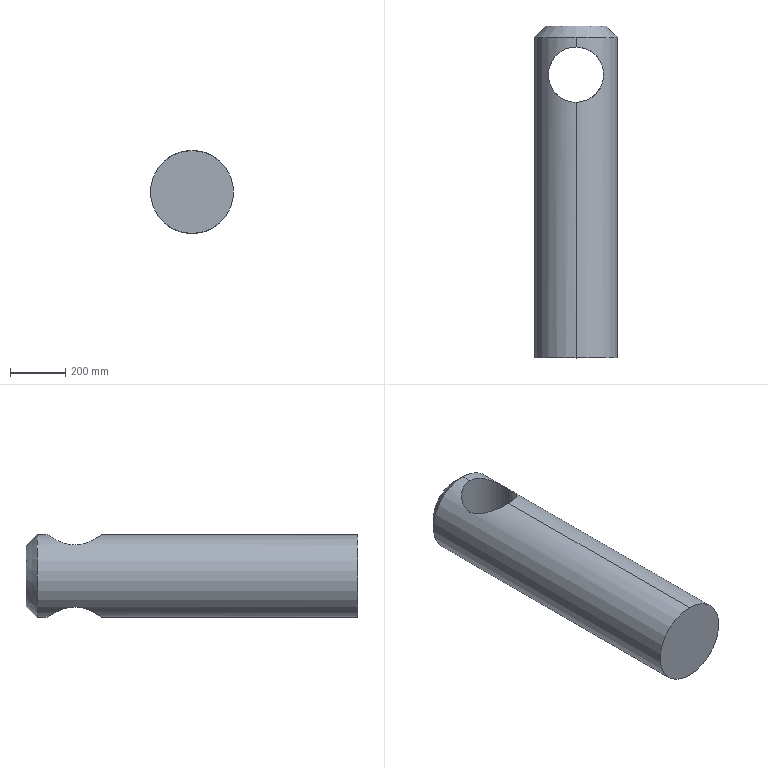Part | SolidWorks | features ICE 2, Chamfer 1, Extrusion 1 | 1 solid | 8 faces | box 300 x 1200 x 300 mm | volume 75269036 mm3 | cylinder 4 | cone 2 | plane 2 | commonest cylinder face diameters 200 x2 300 x2
STEP:
#1=CARTESIAN_POINT('',(0.,2400.,110.));
#2=VERTEX_POINT('',#1);
#3=CARTESIAN_POINT('',(0.,2400.,-110.));
#4=VERTEX_POINT('',#3);
#5=CARTESIAN_POINT('',(0.,2400.,0.));
#6=DIRECTION('',(0.,1.,0.));
#7=DIRECTION('',(0.,0.,1.));
#8=AXIS2_PLACEMENT_3D('',#5,#6,#7);
#9=CIRCLE('',#8,110.);
#10=EDGE_CURVE('',#2,#4,#9,.T.);
#11=ORIENTED_EDGE('',*,*,#10,.F.);
#12=CARTESIAN_POINT('',(0.,2360.,150.));
#13=VERTEX_POINT('',#12);
#14=CARTESIAN_POINT('',(0.,2400.,110.));
#15=DIRECTION('',(0.,-0.7071,0.7071));
#16=VECTOR('',#15,1000.);
#17=LINE('',#14,#16);
#18=EDGE_CURVE('',#2,#13,#17,.T.);
#19=ORIENTED_EDGE('',*,*,#18,.T.);
#20=CARTESIAN_POINT('',(0.,2360.,-150.));
#21=VERTEX_POINT('',#20);
#22=CARTESIAN_POINT('',(0.,2360.,0.));
#23=DIRECTION('',(0.,-1.,0.));
#24=DIRECTION('',(0.,0.,1.));
#25=AXIS2_PLACEMENT_3D('',#22,#23,#24);
#26=CIRCLE('',#25,150.);
#27=EDGE_CURVE('',#21,#13,#26,.T.);
#28=ORIENTED_EDGE('',*,*,#27,.F.);
#29=CARTESIAN_POINT('',(0.,2400.,-110.));
#30=DIRECTION('',(0.,-0.7071,-0.7071));
#31=VECTOR('',#30,1000.);
#32=LINE('',#29,#31);
#33=EDGE_CURVE('',#4,#21,#32,.T.);
#34=ORIENTED_EDGE('',*,*,#33,.F.);
#35=EDGE_LOOP('',(#11,#19,#28,#34));
#36=FACE_OUTER_BOUND('',#35,.T.);
#37=CARTESIAN_POINT('',(0.,2400.,0.));
#38=DIRECTION('',(0.,-1.,0.));
#39=DIRECTION('',(0.,0.,-1.));
#40=AXIS2_PLACEMENT_3D('',#37,#38,#39);
#41=CONICAL_SURFACE('',#40,110.,0.7854);
#42=ADVANCED_FACE('',(#36),#41,.T.);
#43=CARTESIAN_POINT('',(0.,2124.224,150.));
#44=VERTEX_POINT('',#43);
#45=CARTESIAN_POINT('',(100.,2224.224,111.803));
#46=VERTEX_POINT('',#45);
#47=CARTESIAN_POINT('',(0.,2124.224,150.));
#48=CARTESIAN_POINT('',(0.8516,2124.224,150.));
#49=CARTESIAN_POINT('',(1.707,2124.235,149.993));
#50=CARTESIAN_POINT('',(3.415,2124.278,149.964));
#51=CARTESIAN_POINT('',(4.266,2124.311,149.942));
#52=CARTESIAN_POINT('',(6.812,2124.441,149.855));
#53=CARTESIAN_POINT('',(8.499,2124.571,149.768));
#54=CARTESIAN_POINT('',(13.531,2125.086,149.426));
#55=CARTESIAN_POINT('',(16.847,2125.596,149.088));
#56=CARTESIAN_POINT('',(23.402,2126.943,148.2));
#57=CARTESIAN_POINT('',(26.641,2127.779,147.651));
#58=CARTESIAN_POINT('',(31.443,2129.281,146.676));
#59=CARTESIAN_POINT('',(33.023,2129.819,146.328));
#60=CARTESIAN_POINT('',(36.134,2130.965,145.592));
#61=CARTESIAN_POINT('',(37.666,2131.574,145.202));
#62=CARTESIAN_POINT('',(42.196,2133.503,143.977));
#63=CARTESIAN_POINT('',(45.127,2134.926,143.082));
#64=CARTESIAN_POINT('',(49.399,2137.262,141.64));
#65=CARTESIAN_POINT('',(50.802,2138.074,141.143));
#66=CARTESIAN_POINT('',(52.876,2139.342,140.374));
#67=CARTESIAN_POINT('',(53.562,2139.774,140.113));
#68=CARTESIAN_POINT('',(54.923,2140.653,139.585));
#69=CARTESIAN_POINT('',(55.599,2141.101,139.317));
#70=CARTESIAN_POINT('',(58.939,2143.374,137.966));
#71=CARTESIAN_POINT('',(61.492,2145.301,136.843));
#72=CARTESIAN_POINT('',(66.379,2149.365,134.54));
#73=CARTESIAN_POINT('',(68.713,2151.501,133.36));
#74=CARTESIAN_POINT('',(73.171,2155.989,130.967));
#75=CARTESIAN_POINT('',(75.295,2158.339,129.754));
#76=CARTESIAN_POINT('',(78.326,2162.034,127.931));
#77=CARTESIAN_POINT('',(79.306,2163.289,127.326));
#78=CARTESIAN_POINT('',(81.199,2165.835,126.127));
#79=CARTESIAN_POINT('',(82.114,2167.129,125.533));
#80=CARTESIAN_POINT('',(84.762,2171.069,123.774));
#81=CARTESIAN_POINT('',(86.402,2173.777,122.631));
#82=CARTESIAN_POINT('',(89.431,2179.366,120.439));
#83=CARTESIAN_POINT('',(90.821,2182.248,119.39));
#84=CARTESIAN_POINT('',(92.713,2186.715,117.919));
#85=CARTESIAN_POINT('',(93.312,2188.229,117.446));
#86=CARTESIAN_POINT('',(94.442,2191.308,116.539));
#87=CARTESIAN_POINT('',(94.975,2192.879,116.104));
#88=CARTESIAN_POINT('',(96.453,2197.619,114.885));
#89=CARTESIAN_POINT('',(97.281,2200.827,114.18));
#90=CARTESIAN_POINT('',(98.622,2207.348,113.024));
#91=CARTESIAN_POINT('',(99.134,2210.66,112.573));
#92=CARTESIAN_POINT('',(99.565,2214.87,112.191));
#93=CARTESIAN_POINT('',(99.641,2215.716,112.123));
#94=CARTESIAN_POINT('',(99.772,2217.415,112.007));
#95=CARTESIAN_POINT('',(99.826,2218.269,111.959));
#96=CARTESIAN_POINT('',(99.957,2220.829,111.842));
#97=CARTESIAN_POINT('',(100.,2222.529,111.803));
#98=CARTESIAN_POINT('',(100.,2224.224,111.803));
#99=B_SPLINE_CURVE_WITH_KNOTS('',3,(#47,#48,#49,#50,#51,#52,#53,#54,#55,#56,#57,#58,#59,#60,#61,#62,#63,#64,#65,#66,#67,#68,#69,#70,#71,#72,#73,#74,#75,#76,#77,#78,#79,#80,#81,#82,#83,#84,#85,#86,#87,#88,#89,#90,#91,#92,#93,#94,#95,#96,#97,#98),.UNSPECIFIED.,.F.,.F.,(4,2,2,2,2,2,2,2,2,2,2,2,2,2,2,2,2,2,2,2,2,2,2,2,2,4),(0.1618,0.1643,0.1668,0.1718,0.1819,0.192,0.197,0.2021,0.2121,0.2172,0.2197,0.2222,0.2323,0.2424,0.2524,0.2575,0.2625,0.2726,0.2827,0.2877,0.2928,0.3028,0.3129,0.3154,0.3179,0.323),.UNSPECIFIED.);
#100=EDGE_CURVE('',#44,#46,#99,.T.);
#101=ORIENTED_EDGE('',*,*,#100,.T.);
#102=CARTESIAN_POINT('',(100.,2224.224,-111.803));
#103=VERTEX_POINT('',#102);
#104=CARTESIAN_POINT('',(100.,2224.224,4000.));
#105=DIRECTION('',(0.,0.,-1.));
#106=VECTOR('',#105,1000.);
#107=LINE('',#104,#106);
#108=EDGE_CURVE('',#46,#103,#107,.T.);
#109=ORIENTED_EDGE('',*,*,#108,.T.);
#110=CARTESIAN_POINT('',(0.,2124.224,-150.));
#111=VERTEX_POINT('',#110);
#112=CARTESIAN_POINT('',(100.,2224.224,-111.803));
#113=CARTESIAN_POINT('',(100.,2220.834,-111.803));
#114=CARTESIAN_POINT('',(99.828,2217.468,-111.958));
#115=CARTESIAN_POINT('',(99.15,2210.785,-112.559));
#116=CARTESIAN_POINT('',(98.643,2207.467,-113.006));
#117=CARTESIAN_POINT('',(97.8,2203.348,-113.733));
#118=CARTESIAN_POINT('',(97.621,2202.525,-113.887));
#119=CARTESIAN_POINT('',(97.244,2200.892,-114.209));
#120=CARTESIAN_POINT('',(97.045,2200.08,-114.378));
#121=CARTESIAN_POINT('',(96.422,2197.662,-114.904));
#122=CARTESIAN_POINT('',(95.97,2196.072,-115.283));
#123=CARTESIAN_POINT('',(94.502,2191.358,-116.494));
#124=CARTESIAN_POINT('',(93.379,2188.294,-117.401));
#125=CARTESIAN_POINT('',(91.483,2183.806,-118.876));
#126=CARTESIAN_POINT('',(90.815,2182.328,-119.388));
#127=CARTESIAN_POINT('',(89.76,2180.136,-120.18));
#128=CARTESIAN_POINT('',(89.4,2179.409,-120.449));
#129=CARTESIAN_POINT('',(88.663,2177.97,-120.992));
#130=CARTESIAN_POINT('',(88.288,2177.256,-121.266));
#131=CARTESIAN_POINT('',(86.371,2173.723,-122.652));
#132=CARTESIAN_POINT('',(84.718,2170.998,-123.804));
#133=CARTESIAN_POINT('',(81.175,2165.736,-126.156));
#134=CARTESIAN_POINT('',(79.284,2163.199,-127.356));
#135=CARTESIAN_POINT('',(76.266,2159.525,-129.17));
#136=CARTESIAN_POINT('',(75.23,2158.322,-129.777));
#137=CARTESIAN_POINT('',(73.095,2155.962,-130.991));
#138=CARTESIAN_POINT('',(71.995,2154.803,-131.599));
#139=CARTESIAN_POINT('',(68.631,2151.423,-133.403));
#140=CARTESIAN_POINT('',(66.291,2149.287,-134.584));
#141=CARTESIAN_POINT('',(61.415,2145.241,-136.878));
#142=CARTESIAN_POINT('',(58.878,2143.331,-137.991));
#143=CARTESIAN_POINT('',(53.596,2139.739,-140.127));
#144=CARTESIAN_POINT('',(50.851,2138.057,-141.15));
#145=CARTESIAN_POINT('',(47.278,2136.102,-142.356));
#146=CARTESIAN_POINT('',(46.557,2135.719,-142.594));
#147=CARTESIAN_POINT('',(45.099,2134.967,-143.062));
#148=CARTESIAN_POINT('',(44.362,2134.598,-143.292));
#149=CARTESIAN_POINT('',(42.139,2133.521,-143.968));
#150=CARTESIAN_POINT('',(40.641,2132.84,-144.398));
#151=CARTESIAN_POINT('',(36.098,2130.908,-145.625));
#152=CARTESIAN_POINT('',(33.004,2129.769,-146.36));
#153=CARTESIAN_POINT('',(26.679,2127.791,-147.644));
#154=CARTESIAN_POINT('',(23.448,2126.953,-148.193));
#155=CARTESIAN_POINT('',(19.319,2126.104,-148.753));
#156=CARTESIAN_POINT('',(18.488,2125.944,-148.859));
#157=CARTESIAN_POINT('',(16.818,2125.644,-149.057));
#158=CARTESIAN_POINT('',(15.977,2125.505,-149.149));
#159=CARTESIAN_POINT('',(13.458,2125.119,-149.405));
#160=CARTESIAN_POINT('',(11.778,2124.905,-149.546));
#161=CARTESIAN_POINT('',(6.735,2124.393,-149.887));
#162=CARTESIAN_POINT('',(3.369,2124.224,-150.));
#163=CARTESIAN_POINT('',(0.,2124.224,-150.));
#164=B_SPLINE_CURVE_WITH_KNOTS('',3,(#112,#113,#114,#115,#116,#117,#118,#119,#120,#121,#122,#123,#124,#125,#126,#127,#128,#129,#130,#131,#132,#133,#134,#135,#136,#137,#138,#139,#140,#141,#142,#143,#144,#145,#146,#147,#148,#149,#150,#151,#152,#153,#154,#155,#156,#157,#158,#159,#160,#161,#162,#163),.UNSPECIFIED.,.F.,.F.,(4,2,2,2,2,2,2,2,2,2,2,2,2,2,2,2,2,2,2,2,2,2,2,2,2,4),(0.1617,0.1718,0.1819,0.1844,0.1869,0.192,0.2021,0.2071,0.2096,0.2122,0.2223,0.2323,0.2374,0.2424,0.2525,0.2626,0.2727,0.2752,0.2778,0.2828,0.2929,0.303,0.3055,0.3081,0.3131,0.3232),.UNSPECIFIED.);
#165=EDGE_CURVE('',#103,#111,#164,.T.);
#166=ORIENTED_EDGE('',*,*,#165,.T.);
#167=CARTESIAN_POINT('',(-100.,2224.224,-111.803));
#168=VERTEX_POINT('',#167);
#169=CARTESIAN_POINT('',(0.,2124.224,-150.));
#170=CARTESIAN_POINT('',(-3.365,2124.224,-150.));
#171=CARTESIAN_POINT('',(-6.734,2124.393,-149.887));
#172=CARTESIAN_POINT('',(-10.949,2124.821,-149.602));
#173=CARTESIAN_POINT('',(-11.792,2124.918,-149.538));
#174=CARTESIAN_POINT('',(-13.479,2125.133,-149.396));
#175=CARTESIAN_POINT('',(-14.324,2125.251,-149.317));
#176=CARTESIAN_POINT('',(-16.84,2125.637,-149.061));
#177=CARTESIAN_POINT('',(-18.501,2125.936,-148.864));
#178=CARTESIAN_POINT('',(-23.436,2126.951,-148.195));
#179=CARTESIAN_POINT('',(-26.662,2127.786,-147.647));
#180=CARTESIAN_POINT('',(-32.993,2129.765,-146.362));
#181=CARTESIAN_POINT('',(-36.097,2130.907,-145.626));
#182=CARTESIAN_POINT('',(-39.904,2132.526,-144.597));
#183=CARTESIAN_POINT('',(-40.662,2132.86,-144.386));
#184=CARTESIAN_POINT('',(-42.164,2133.544,-143.954));
#185=CARTESIAN_POINT('',(-42.908,2133.893,-143.734));
#186=CARTESIAN_POINT('',(-45.121,2134.967,-143.061));
#187=CARTESIAN_POINT('',(-46.57,2135.715,-142.596));
#188=CARTESIAN_POINT('',(-50.841,2138.051,-141.153));
#189=CARTESIAN_POINT('',(-53.588,2139.734,-140.13));
#190=CARTESIAN_POINT('',(-58.893,2143.342,-137.985));
#191=CARTESIAN_POINT('',(-61.451,2145.267,-136.862));
#192=CARTESIAN_POINT('',(-65.15,2148.342,-135.12));
#193=CARTESIAN_POINT('',(-66.356,2149.394,-134.531));
#194=CARTESIAN_POINT('',(-68.703,2151.543,-133.348));
#195=CARTESIAN_POINT('',(-69.847,2152.642,-132.752));
#196=CARTESIAN_POINT('',(-73.19,2156.009,-130.957));
#197=CARTESIAN_POINT('',(-75.302,2158.348,-129.75));
#198=CARTESIAN_POINT('',(-79.302,2163.223,-127.345));
#199=CARTESIAN_POINT('',(-81.19,2165.758,-126.146));
#200=CARTESIAN_POINT('',(-83.855,2169.718,-124.376));
#201=CARTESIAN_POINT('',(-84.716,2171.065,-123.791));
#202=CARTESIAN_POINT('',(-86.379,2173.813,-122.637));
#203=CARTESIAN_POINT('',(-87.176,2175.204,-122.071));
#204=CARTESIAN_POINT('',(-89.466,2179.434,-120.413));
#205=CARTESIAN_POINT('',(-90.858,2182.328,-119.362));
#206=CARTESIAN_POINT('',(-93.37,2188.274,-117.407));
#207=CARTESIAN_POINT('',(-94.491,2191.327,-116.503));
#208=CARTESIAN_POINT('',(-95.96,2196.04,-115.291));
#209=CARTESIAN_POINT('',(-96.414,2197.633,-114.911));
#210=CARTESIAN_POINT('',(-97.04,2200.06,-114.382));
#211=CARTESIAN_POINT('',(-97.24,2200.875,-114.213));
#212=CARTESIAN_POINT('',(-97.617,2202.508,-113.89));
#213=CARTESIAN_POINT('',(-97.796,2203.326,-113.737));
#214=CARTESIAN_POINT('',(-98.636,2207.428,-113.012));
#215=CARTESIAN_POINT('',(-99.144,2210.74,-112.564));
#216=CARTESIAN_POINT('',(-99.826,2217.431,-111.96));
#217=CARTESIAN_POINT('',(-100.,2220.81,-111.803));
#218=CARTESIAN_POINT('',(-100.,2224.224,-111.803));
#219=B_SPLINE_CURVE_WITH_KNOTS('',3,(#169,#170,#171,#172,#173,#174,#175,#176,#177,#178,#179,#180,#181,#182,#183,#184,#185,#186,#187,#188,#189,#190,#191,#192,#193,#194,#195,#196,#197,#198,#199,#200,#201,#202,#203,#204,#205,#206,#207,#208,#209,#210,#211,#212,#213,#214,#215,#216,#217,#218),.UNSPECIFIED.,.F.,.F.,(4,2,2,2,2,2,2,2,2,2,2,2,2,2,2,2,2,2,2,2,2,2,2,2,4),(0.3232,0.3333,0.3358,0.3383,0.3434,0.3534,0.3635,0.366,0.3686,0.3736,0.3837,0.3938,0.3988,0.4039,0.4139,0.424,0.4291,0.4341,0.4442,0.4543,0.4593,0.4618,0.4644,0.4744,0.4845),.UNSPECIFIED.);
#220=EDGE_CURVE('',#111,#168,#219,.T.);
#221=ORIENTED_EDGE('',*,*,#220,.T.);
#222=CARTESIAN_POINT('',(-100.,2224.224,111.803));
#223=VERTEX_POINT('',#222);
#224=CARTESIAN_POINT('',(-100.,2224.224,4000.));
#225=DIRECTION('',(0.,0.,-1.));
#226=VECTOR('',#225,1000.);
#227=LINE('',#224,#226);
#228=EDGE_CURVE('',#223,#168,#227,.T.);
#229=ORIENTED_EDGE('',*,*,#228,.F.);
#230=CARTESIAN_POINT('',(-100.,2224.224,111.803));
#231=CARTESIAN_POINT('',(-100.,2220.792,111.803));
#232=CARTESIAN_POINT('',(-99.824,2217.405,111.962));
#233=CARTESIAN_POINT('',(-99.141,2210.717,112.567));
#234=CARTESIAN_POINT('',(-98.634,2207.416,113.014));
#235=CARTESIAN_POINT('',(-97.631,2202.523,113.879));
#236=CARTESIAN_POINT('',(-97.257,2200.902,114.199));
#237=CARTESIAN_POINT('',(-96.635,2198.486,114.725));
#238=CARTESIAN_POINT('',(-96.417,2197.682,114.908));
#239=CARTESIAN_POINT('',(-95.962,2196.081,115.288));
#240=CARTESIAN_POINT('',(-95.724,2195.282,115.486));
#241=CARTESIAN_POINT('',(-94.49,2191.319,116.505));
#242=CARTESIAN_POINT('',(-93.361,2188.248,117.415));
#243=CARTESIAN_POINT('',(-90.834,2182.276,119.38));
#244=CARTESIAN_POINT('',(-89.437,2179.376,120.435));
#245=CARTESIAN_POINT('',(-87.143,2175.145,122.095));
#246=CARTESIAN_POINT('',(-86.344,2173.754,122.661));
#247=CARTESIAN_POINT('',(-84.681,2171.01,123.815));
#248=CARTESIAN_POINT('',(-83.814,2169.655,124.404));
#249=CARTESIAN_POINT('',(-81.135,2165.681,126.181));
#250=CARTESIAN_POINT('',(-79.238,2163.139,127.385));
#251=CARTESIAN_POINT('',(-75.221,2158.255,129.797));
#252=CARTESIAN_POINT('',(-73.101,2155.914,131.006));
#253=CARTESIAN_POINT('',(-68.63,2151.423,133.403));
#254=CARTESIAN_POINT('',(-66.28,2149.275,134.59));
#255=CARTESIAN_POINT('',(-62.567,2146.199,136.335));
#256=CARTESIAN_POINT('',(-61.306,2145.204,136.907));
#257=CARTESIAN_POINT('',(-58.743,2143.28,138.026));
#258=CARTESIAN_POINT('',(-57.439,2142.35,138.574));
#259=CARTESIAN_POINT('',(-53.463,2139.655,140.178));
#260=CARTESIAN_POINT('',(-50.725,2137.984,141.194));
#261=CARTESIAN_POINT('',(-45.067,2134.896,143.101));
#262=CARTESIAN_POINT('',(-42.146,2133.48,143.991));
#263=CARTESIAN_POINT('',(-37.617,2131.554,145.215));
#264=CARTESIAN_POINT('',(-36.083,2130.946,145.604));
#265=CARTESIAN_POINT('',(-33.743,2130.085,146.158));
#266=CARTESIAN_POINT('',(-32.956,2129.807,146.337));
#267=CARTESIAN_POINT('',(-31.37,2129.268,146.685));
#268=CARTESIAN_POINT('',(-30.57,2129.007,146.854));
#269=CARTESIAN_POINT('',(-26.569,2127.759,147.664));
#270=CARTESIAN_POINT('',(-23.332,2126.926,148.211));
#271=CARTESIAN_POINT('',(-16.789,2125.587,149.094));
#272=CARTESIAN_POINT('',(-13.482,2125.08,149.43));
#273=CARTESIAN_POINT('',(-6.796,2124.398,149.883));
#274=CARTESIAN_POINT('',(-3.417,2124.224,150.));
#275=CARTESIAN_POINT('',(0.,2124.224,150.));
#276=B_SPLINE_CURVE_WITH_KNOTS('',3,(#230,#231,#232,#233,#234,#235,#236,#237,#238,#239,#240,#241,#242,#243,#244,#245,#246,#247,#248,#249,#250,#251,#252,#253,#254,#255,#256,#257,#258,#259,#260,#261,#262,#263,#264,#265,#266,#267,#268,#269,#270,#271,#272,#273,#274,#275),.UNSPECIFIED.,.F.,.F.,(4,2,2,2,2,2,2,2,2,2,2,2,2,2,2,2,2,2,2,2,2,2,4),(0.,0.01011,0.02022,0.02527,0.0278,0.03033,0.04044,0.05055,0.0556,0.06066,0.07077,0.08088,0.09099,0.09604,0.1011,0.1112,0.1213,0.1264,0.1289,0.1314,0.1415,0.1516,0.1618),.UNSPECIFIED.);
#277=EDGE_CURVE('',#223,#44,#276,.T.);
#278=ORIENTED_EDGE('',*,*,#277,.T.);
#279=EDGE_LOOP('',(#101,#109,#166,#221,#229,#278));
#280=FACE_OUTER_BOUND('',#279,.T.);
#281=CARTESIAN_POINT('',(0.,2224.224,4000.));
#282=DIRECTION('',(0.,0.,-1.));
#283=DIRECTION('',(-1.,0.,0.));
#284=AXIS2_PLACEMENT_3D('',#281,#282,#283);
#285=CYLINDRICAL_SURFACE('',#284,100.);
#286=ADVANCED_FACE('',(#280),#285,.F.);
#287=ORIENTED_EDGE('',*,*,#27,.T.);
#288=CARTESIAN_POINT('',(0.,2324.224,150.));
#289=VERTEX_POINT('',#288);
#290=CARTESIAN_POINT('',(0.,2400.,150.));
#291=DIRECTION('',(0.,-1.,0.));
#292=VECTOR('',#291,1000.);
#293=LINE('',#290,#292);
#294=EDGE_CURVE('',#13,#289,#293,.T.);
#295=ORIENTED_EDGE('',*,*,#294,.T.);
#296=CARTESIAN_POINT('',(100.,2224.224,111.803));
#297=CARTESIAN_POINT('',(100.,2227.611,111.803));
#298=CARTESIAN_POINT('',(99.828,2230.975,111.958));
#299=CARTESIAN_POINT('',(99.15,2237.659,112.559));
#300=CARTESIAN_POINT('',(98.644,2240.979,113.005));
#301=CARTESIAN_POINT('',(97.8,2245.102,113.733));
#302=CARTESIAN_POINT('',(97.621,2245.925,113.887));
#303=CARTESIAN_POINT('',(97.243,2247.557,114.209));
#304=CARTESIAN_POINT('',(97.045,2248.368,114.378));
#305=CARTESIAN_POINT('',(96.423,2250.784,114.904));
#306=CARTESIAN_POINT('',(95.97,2252.375,115.283));
#307=CARTESIAN_POINT('',(94.503,2257.087,116.494));
#308=CARTESIAN_POINT('',(93.38,2260.151,117.4));
#309=CARTESIAN_POINT('',(91.482,2264.641,118.876));
#310=CARTESIAN_POINT('',(90.815,2266.12,119.388));
#311=CARTESIAN_POINT('',(89.759,2268.313,120.181));
#312=CARTESIAN_POINT('',(89.399,2269.04,120.45));
#313=CARTESIAN_POINT('',(88.663,2270.479,120.992));
#314=CARTESIAN_POINT('',(88.287,2271.192,121.267));
#315=CARTESIAN_POINT('',(86.372,2274.724,122.652));
#316=CARTESIAN_POINT('',(84.719,2277.448,123.803));
#317=CARTESIAN_POINT('',(81.175,2282.71,126.155));
#318=CARTESIAN_POINT('',(79.285,2285.248,127.356));
#319=CARTESIAN_POINT('',(76.265,2288.924,129.17));
#320=CARTESIAN_POINT('',(75.228,2290.127,129.778));
#321=CARTESIAN_POINT('',(73.625,2291.899,130.689));
#322=CARTESIAN_POINT('',(73.083,2292.485,130.994));
#323=CARTESIAN_POINT('',(71.986,2293.64,131.599));
#324=CARTESIAN_POINT('',(71.432,2294.21,131.901));
#325=CARTESIAN_POINT('',(68.631,2297.024,133.403));
#326=CARTESIAN_POINT('',(66.292,2299.159,134.583));
#327=CARTESIAN_POINT('',(61.417,2303.205,136.877));
#328=CARTESIAN_POINT('',(58.88,2305.115,137.99));
#329=CARTESIAN_POINT('',(53.596,2308.709,140.127));
#330=CARTESIAN_POINT('',(50.849,2310.392,141.151));
#331=CARTESIAN_POINT('',(47.272,2312.349,142.359));
#332=CARTESIAN_POINT('',(46.549,2312.733,142.597));
#333=CARTESIAN_POINT('',(45.089,2313.485,143.065));
#334=CARTESIAN_POINT('',(44.352,2313.854,143.295));
#335=CARTESIAN_POINT('',(42.132,2314.93,143.97));
#336=CARTESIAN_POINT('',(40.636,2315.61,144.399));
#337=CARTESIAN_POINT('',(36.096,2317.54,145.626));
#338=CARTESIAN_POINT('',(33.003,2318.679,146.36));
#339=CARTESIAN_POINT('',(26.677,2320.657,147.644));
#340=CARTESIAN_POINT('',(23.445,2321.495,148.194));
#341=CARTESIAN_POINT('',(19.311,2322.345,148.754));
#342=CARTESIAN_POINT('',(18.479,2322.505,148.86));
#343=CARTESIAN_POINT('',(16.807,2322.805,149.058));
#344=CARTESIAN_POINT('',(15.967,2322.944,149.15));
#345=CARTESIAN_POINT('',(13.452,2323.329,149.405));
#346=CARTESIAN_POINT('',(11.773,2323.543,149.547));
#347=CARTESIAN_POINT('',(6.734,2324.054,149.887));
#348=CARTESIAN_POINT('',(3.369,2324.224,150.));
#349=CARTESIAN_POINT('',(0.,2324.224,150.));
#350=B_SPLINE_CURVE_WITH_KNOTS('',3,(#296,#297,#298,#299,#300,#301,#302,#303,#304,#305,#306,#307,#308,#309,#310,#311,#312,#313,#314,#315,#316,#317,#318,#319,#320,#321,#322,#323,#324,#325,#326,#327,#328,#329,#330,#331,#332,#333,#334,#335,#336,#337,#338,#339,#340,#341,#342,#343,#344,#345,#346,#347,#348,#349),.UNSPECIFIED.,.F.,.F.,(4,2,2,2,2,2,2,2,2,2,2,2,2,2,2,2,2,2,2,2,2,2,2,2,2,2,4),(0.323,0.3331,0.3431,0.3456,0.3482,0.3532,0.3633,0.3683,0.3708,0.3733,0.3834,0.3935,0.3985,0.401,0.4035,0.4136,0.4237,0.4338,0.4363,0.4388,0.4438,0.4539,0.464,0.4665,0.469,0.474,0.4841),.UNSPECIFIED.);
#351=EDGE_CURVE('',#46,#289,#350,.T.);
#352=ORIENTED_EDGE('',*,*,#351,.F.);
#353=ORIENTED_EDGE('',*,*,#100,.F.);
#354=CARTESIAN_POINT('',(0.,1200.,150.));
#355=VERTEX_POINT('',#354);
#356=CARTESIAN_POINT('',(0.,2400.,150.));
#357=DIRECTION('',(0.,-1.,0.));
#358=VECTOR('',#357,1000.);
#359=LINE('',#356,#358);
#360=EDGE_CURVE('',#44,#355,#359,.T.);
#361=ORIENTED_EDGE('',*,*,#360,.T.);
#362=CARTESIAN_POINT('',(0.,1200.,-150.));
#363=VERTEX_POINT('',#362);
#364=CARTESIAN_POINT('',(0.,1200.,0.));
#365=DIRECTION('',(0.,-1.,0.));
#366=DIRECTION('',(0.,0.,-1.));
#367=AXIS2_PLACEMENT_3D('',#364,#365,#366);
#368=CIRCLE('',#367,150.);
#369=EDGE_CURVE('',#363,#355,#368,.T.);
#370=ORIENTED_EDGE('',*,*,#369,.F.);
#371=CARTESIAN_POINT('',(0.,2400.,-150.));
#372=DIRECTION('',(0.,-1.,0.));
#373=VECTOR('',#372,1000.);
#374=LINE('',#371,#373);
#375=EDGE_CURVE('',#111,#363,#374,.T.);
#376=ORIENTED_EDGE('',*,*,#375,.F.);
#377=ORIENTED_EDGE('',*,*,#165,.F.);
#378=CARTESIAN_POINT('',(0.,2324.224,-150.));
#379=VERTEX_POINT('',#378);
#380=CARTESIAN_POINT('',(0.,2324.224,-150.));
#381=CARTESIAN_POINT('',(3.423,2324.224,-150.));
#382=CARTESIAN_POINT('',(6.808,2324.048,-149.883));
#383=CARTESIAN_POINT('',(13.506,2323.365,-149.428));
#384=CARTESIAN_POINT('',(16.818,2322.856,-149.091));
#385=CARTESIAN_POINT('',(21.734,2321.847,-148.426));
#386=CARTESIAN_POINT('',(23.364,2321.47,-148.178));
#387=CARTESIAN_POINT('',(26.607,2320.634,-147.631));
#388=CARTESIAN_POINT('',(28.221,2320.174,-147.33));
#389=CARTESIAN_POINT('',(33.026,2318.672,-146.356));
#390=CARTESIAN_POINT('',(36.133,2317.525,-145.617));
#391=CARTESIAN_POINT('',(42.17,2314.957,-143.984));
#392=CARTESIAN_POINT('',(45.1,2313.535,-143.091));
#393=CARTESIAN_POINT('',(49.37,2311.202,-141.65));
#394=CARTESIAN_POINT('',(50.773,2310.391,-141.153));
#395=CARTESIAN_POINT('',(52.846,2309.124,-140.385));
#396=CARTESIAN_POINT('',(53.532,2308.693,-140.125));
#397=CARTESIAN_POINT('',(54.893,2307.814,-139.597));
#398=CARTESIAN_POINT('',(55.569,2307.366,-139.329));
#399=CARTESIAN_POINT('',(58.914,2305.092,-137.976));
#400=CARTESIAN_POINT('',(61.47,2303.164,-136.853));
#401=CARTESIAN_POINT('',(66.361,2299.099,-134.549));
#402=CARTESIAN_POINT('',(68.696,2296.962,-133.369));
#403=CARTESIAN_POINT('',(73.155,2292.475,-130.976));
#404=CARTESIAN_POINT('',(75.28,2290.126,-129.763));
#405=CARTESIAN_POINT('',(77.805,2287.049,-128.245));
#406=CARTESIAN_POINT('',(78.304,2286.426,-127.941));
#407=CARTESIAN_POINT('',(79.285,2285.171,-127.335));
#408=CARTESIAN_POINT('',(79.767,2284.539,-127.034));
#409=CARTESIAN_POINT('',(81.188,2282.627,-126.134));
#410=CARTESIAN_POINT('',(82.104,2281.333,-125.539));
#411=CARTESIAN_POINT('',(84.755,2277.39,-123.779));
#412=CARTESIAN_POINT('',(86.395,2274.681,-122.635));
#413=CARTESIAN_POINT('',(89.426,2269.091,-120.443));
#414=CARTESIAN_POINT('',(90.816,2266.21,-119.394));
#415=CARTESIAN_POINT('',(92.708,2261.744,-117.923));
#416=CARTESIAN_POINT('',(93.306,2260.232,-117.45));
#417=CARTESIAN_POINT('',(94.154,2257.924,-116.77));
#418=CARTESIAN_POINT('',(94.428,2257.148,-116.548));
#419=CARTESIAN_POINT('',(94.959,2255.584,-116.116));
#420=CARTESIAN_POINT('',(95.216,2254.794,-115.905));
#421=CARTESIAN_POINT('',(96.45,2250.839,-114.887));
#422=CARTESIAN_POINT('',(97.28,2247.627,-114.182));
#423=CARTESIAN_POINT('',(98.621,2241.104,-113.025));
#424=CARTESIAN_POINT('',(99.133,2237.791,-112.574));
#425=CARTESIAN_POINT('',(99.651,2232.741,-112.115));
#426=CARTESIAN_POINT('',(99.782,2231.042,-111.998));
#427=CARTESIAN_POINT('',(99.957,2227.623,-111.842));
#428=CARTESIAN_POINT('',(100.,2225.92,-111.803));
#429=CARTESIAN_POINT('',(100.,2224.224,-111.803));
#430=B_SPLINE_CURVE_WITH_KNOTS('',3,(#380,#381,#382,#383,#384,#385,#386,#387,#388,#389,#390,#391,#392,#393,#394,#395,#396,#397,#398,#399,#400,#401,#402,#403,#404,#405,#406,#407,#408,#409,#410,#411,#412,#413,#414,#415,#416,#417,#418,#419,#420,#421,#422,#423,#424,#425,#426,#427,#428,#429),.UNSPECIFIED.,.F.,.F.,(4,2,2,2,2,2,2,2,2,2,2,2,2,2,2,2,2,2,2,2,2,2,2,2,4),(0.,0.01011,0.02021,0.02526,0.03032,0.04042,0.05053,0.05558,0.05811,0.06063,0.07074,0.08084,0.09095,0.09347,0.096,0.1011,0.1112,0.1213,0.1263,0.1288,0.1314,0.1415,0.1516,0.1566,0.1617),.UNSPECIFIED.);
#431=EDGE_CURVE('',#379,#103,#430,.T.);
#432=ORIENTED_EDGE('',*,*,#431,.F.);
#433=CARTESIAN_POINT('',(0.,2400.,-150.));
#434=DIRECTION('',(0.,-1.,0.));
#435=VECTOR('',#434,1000.);
#436=LINE('',#433,#435);
#437=EDGE_CURVE('',#21,#379,#436,.T.);
#438=ORIENTED_EDGE('',*,*,#437,.F.);
#439=EDGE_LOOP('',(#287,#295,#352,#353,#361,#370,#376,#377,#432,#438));
#440=FACE_OUTER_BOUND('',#439,.T.);
#441=CARTESIAN_POINT('',(0.,2400.,0.));
#442=DIRECTION('',(0.,-1.,0.));
#443=DIRECTION('',(0.,0.,-1.));
#444=AXIS2_PLACEMENT_3D('',#441,#442,#443);
#445=CYLINDRICAL_SURFACE('',#444,150.);
#446=ADVANCED_FACE('',(#440),#445,.T.);
#447=ORIENTED_EDGE('',*,*,#294,.F.);
#448=CARTESIAN_POINT('',(0.,2360.,0.));
#449=DIRECTION('',(0.,-1.,0.));
#450=DIRECTION('',(0.,0.,1.));
#451=AXIS2_PLACEMENT_3D('',#448,#449,#450);
#452=CIRCLE('',#451,150.);
#453=EDGE_CURVE('',#13,#21,#452,.T.);
#454=ORIENTED_EDGE('',*,*,#453,.T.);
#455=ORIENTED_EDGE('',*,*,#437,.T.);
#456=CARTESIAN_POINT('',(-100.,2224.224,-111.803));
#457=CARTESIAN_POINT('',(-100.,2225.078,-111.803));
#458=CARTESIAN_POINT('',(-99.989,2225.936,-111.813));
#459=CARTESIAN_POINT('',(-99.945,2227.646,-111.853));
#460=CARTESIAN_POINT('',(-99.912,2228.498,-111.882));
#461=CARTESIAN_POINT('',(-99.781,2231.047,-111.999));
#462=CARTESIAN_POINT('',(-99.651,2232.735,-112.114));
#463=CARTESIAN_POINT('',(-99.136,2237.766,-112.571));
#464=CARTESIAN_POINT('',(-98.626,2241.077,-113.021));
#465=CARTESIAN_POINT('',(-97.618,2245.984,-113.89));
#466=CARTESIAN_POINT('',(-97.241,2247.609,-114.212));
#467=CARTESIAN_POINT('',(-96.407,2250.84,-114.917));
#468=CARTESIAN_POINT('',(-95.948,2252.449,-115.301));
#469=CARTESIAN_POINT('',(-94.469,2257.186,-116.521));
#470=CARTESIAN_POINT('',(-93.343,2260.246,-117.43));
#471=CARTESIAN_POINT('',(-90.823,2266.195,-119.389));
#472=CARTESIAN_POINT('',(-89.431,2269.083,-120.44));
#473=CARTESIAN_POINT('',(-87.145,2273.299,-122.093));
#474=CARTESIAN_POINT('',(-86.35,2274.684,-122.657));
#475=CARTESIAN_POINT('',(-84.694,2277.417,-123.806));
#476=CARTESIAN_POINT('',(-83.832,2278.766,-124.392));
#477=CARTESIAN_POINT('',(-81.149,2282.748,-126.172));
#478=CARTESIAN_POINT('',(-79.25,2285.293,-127.377));
#479=CARTESIAN_POINT('',(-75.234,2290.177,-129.79));
#480=CARTESIAN_POINT('',(-73.117,2292.517,-130.998));
#481=CARTESIAN_POINT('',(-68.656,2297.,-133.39));
#482=CARTESIAN_POINT('',(-66.312,2299.143,-134.574));
#483=CARTESIAN_POINT('',(-62.616,2302.209,-136.312));
#484=CARTESIAN_POINT('',(-61.351,2303.209,-136.887));
#485=CARTESIAN_POINT('',(-58.782,2305.139,-138.009));
#486=CARTESIAN_POINT('',(-57.477,2306.071,-138.559));
#487=CARTESIAN_POINT('',(-53.497,2308.772,-140.165));
#488=CARTESIAN_POINT('',(-50.759,2310.443,-141.182));
#489=CARTESIAN_POINT('',(-45.108,2313.53,-143.088));
#490=CARTESIAN_POINT('',(-42.195,2314.944,-143.977));
#491=CARTESIAN_POINT('',(-36.181,2317.506,-145.605));
#492=CARTESIAN_POINT('',(-33.079,2318.654,-146.344));
#493=CARTESIAN_POINT('',(-29.074,2319.908,-147.158));
#494=CARTESIAN_POINT('',(-28.267,2320.149,-147.315));
#495=CARTESIAN_POINT('',(-26.651,2320.61,-147.616));
#496=CARTESIAN_POINT('',(-25.841,2320.831,-147.76));
#497=CARTESIAN_POINT('',(-23.405,2321.461,-148.172));
#498=CARTESIAN_POINT('',(-21.772,2321.839,-148.421));
#499=CARTESIAN_POINT('',(-16.846,2322.851,-149.088));
#500=CARTESIAN_POINT('',(-13.528,2323.362,-149.427));
#501=CARTESIAN_POINT('',(-8.496,2323.876,-149.769));
#502=CARTESIAN_POINT('',(-6.81,2324.006,-149.855));
#503=CARTESIAN_POINT('',(-4.267,2324.136,-149.942));
#504=CARTESIAN_POINT('',(-3.416,2324.169,-149.964));
#505=CARTESIAN_POINT('',(-2.138,2324.202,-149.985));
#506=CARTESIAN_POINT('',(-1.711,2324.21,-149.991));
#507=CARTESIAN_POINT('',(-0.8565,2324.221,-149.998));
#508=CARTESIAN_POINT('',(-0.4273,2324.224,-150.));
#509=CARTESIAN_POINT('',(0.,2324.224,-150.));
#510=B_SPLINE_CURVE_WITH_KNOTS('',3,(#456,#457,#458,#459,#460,#461,#462,#463,#464,#465,#466,#467,#468,#469,#470,#471,#472,#473,#474,#475,#476,#477,#478,#479,#480,#481,#482,#483,#484,#485,#486,#487,#488,#489,#490,#491,#492,#493,#494,#495,#496,#497,#498,#499,#500,#501,#502,#503,#504,#505,#506,#507,#508,#509),.UNSPECIFIED.,.F.,.F.,(4,2,2,2,2,2,2,2,2,2,2,2,2,2,2,2,2,2,2,2,2,2,2,2,2,2,4),(0.4845,0.487,0.4896,0.4946,0.5047,0.5097,0.5148,0.5249,0.535,0.54,0.5451,0.5552,0.5652,0.5753,0.5804,0.5854,0.5955,0.6056,0.6157,0.6182,0.6207,0.6258,0.6359,0.6409,0.6434,0.6447,0.646),.UNSPECIFIED.);
#511=EDGE_CURVE('',#168,#379,#510,.T.);
#512=ORIENTED_EDGE('',*,*,#511,.F.);
#513=ORIENTED_EDGE('',*,*,#220,.F.);
#514=ORIENTED_EDGE('',*,*,#375,.T.);
#515=CARTESIAN_POINT('',(0.,1200.,0.));
#516=DIRECTION('',(0.,-1.,0.));
#517=DIRECTION('',(0.,0.,-1.));
#518=AXIS2_PLACEMENT_3D('',#515,#516,#517);
#519=CIRCLE('',#518,150.);
#520=EDGE_CURVE('',#355,#363,#519,.T.);
#521=ORIENTED_EDGE('',*,*,#520,.F.);
#522=ORIENTED_EDGE('',*,*,#360,.F.);
#523=ORIENTED_EDGE('',*,*,#277,.F.);
#524=CARTESIAN_POINT('',(0.,2324.224,150.));
#525=CARTESIAN_POINT('',(-3.365,2324.224,150.));
#526=CARTESIAN_POINT('',(-6.734,2324.054,149.887));
#527=CARTESIAN_POINT('',(-10.952,2323.626,149.602));
#528=CARTESIAN_POINT('',(-11.796,2323.529,149.538));
#529=CARTESIAN_POINT('',(-13.485,2323.314,149.395));
#530=CARTESIAN_POINT('',(-14.328,2323.196,149.317));
#531=CARTESIAN_POINT('',(-16.841,2322.81,149.061));
#532=CARTESIAN_POINT('',(-18.501,2322.512,148.864));
#533=CARTESIAN_POINT('',(-23.432,2321.498,148.196));
#534=CARTESIAN_POINT('',(-26.656,2320.662,147.648));
#535=CARTESIAN_POINT('',(-32.987,2318.685,146.364));
#536=CARTESIAN_POINT('',(-36.092,2317.542,145.627));
#537=CARTESIAN_POINT('',(-39.901,2315.922,144.598));
#538=CARTESIAN_POINT('',(-40.659,2315.588,144.386));
#539=CARTESIAN_POINT('',(-42.16,2314.906,143.955));
#540=CARTESIAN_POINT('',(-42.903,2314.556,143.736));
#541=CARTESIAN_POINT('',(-45.114,2313.484,143.063));
#542=CARTESIAN_POINT('',(-46.562,2312.737,142.598));
#543=CARTESIAN_POINT('',(-50.832,2310.402,141.156));
#544=CARTESIAN_POINT('',(-53.578,2308.72,140.134));
#545=CARTESIAN_POINT('',(-58.884,2305.113,137.989));
#546=CARTESIAN_POINT('',(-61.442,2303.187,136.866));
#547=CARTESIAN_POINT('',(-66.377,2299.086,134.542));
#548=CARTESIAN_POINT('',(-68.722,2296.937,133.355));
#549=CARTESIAN_POINT('',(-73.178,2292.451,130.963));
#550=CARTESIAN_POINT('',(-75.29,2290.113,129.757));
#551=CARTESIAN_POINT('',(-79.291,2285.24,127.352));
#552=CARTESIAN_POINT('',(-81.18,2282.705,126.152));
#553=CARTESIAN_POINT('',(-83.402,2279.403,124.677));
#554=CARTESIAN_POINT('',(-83.839,2278.736,124.383));
#555=CARTESIAN_POINT('',(-84.7,2277.389,123.799));
#556=CARTESIAN_POINT('',(-85.124,2276.707,123.508));
#557=CARTESIAN_POINT('',(-86.37,2274.649,122.643));
#558=CARTESIAN_POINT('',(-87.167,2273.259,122.077));
#559=CARTESIAN_POINT('',(-89.456,2269.034,120.421));
#560=CARTESIAN_POINT('',(-90.847,2266.142,119.37));
#561=CARTESIAN_POINT('',(-93.361,2260.199,117.415));
#562=CARTESIAN_POINT('',(-94.482,2257.147,116.511));
#563=CARTESIAN_POINT('',(-95.953,2252.433,115.297));
#564=CARTESIAN_POINT('',(-96.408,2250.839,114.917));
#565=CARTESIAN_POINT('',(-97.034,2248.411,114.387));
#566=CARTESIAN_POINT('',(-97.234,2247.596,114.218));
#567=CARTESIAN_POINT('',(-97.611,2245.965,113.895));
#568=CARTESIAN_POINT('',(-97.79,2245.148,113.742));
#569=CARTESIAN_POINT('',(-98.631,2241.049,113.016));
#570=CARTESIAN_POINT('',(-99.14,2237.735,112.567));
#571=CARTESIAN_POINT('',(-99.653,2232.71,112.113));
#572=CARTESIAN_POINT('',(-99.783,2231.026,111.997));
#573=CARTESIAN_POINT('',(-99.913,2228.486,111.881));
#574=CARTESIAN_POINT('',(-99.945,2227.637,111.852));
#575=CARTESIAN_POINT('',(-99.978,2226.359,111.823));
#576=CARTESIAN_POINT('',(-99.986,2225.933,111.816));
#577=CARTESIAN_POINT('',(-99.997,2225.079,111.806));
#578=CARTESIAN_POINT('',(-100.,2224.65,111.803));
#579=CARTESIAN_POINT('',(-100.,2224.224,111.803));
#580=B_SPLINE_CURVE_WITH_KNOTS('',3,(#524,#525,#526,#527,#528,#529,#530,#531,#532,#533,#534,#535,#536,#537,#538,#539,#540,#541,#542,#543,#544,#545,#546,#547,#548,#549,#550,#551,#552,#553,#554,#555,#556,#557,#558,#559,#560,#561,#562,#563,#564,#565,#566,#567,#568,#569,#570,#571,#572,#573,#574,#575,#576,#577,#578,#579),.UNSPECIFIED.,.F.,.F.,(4,2,2,2,2,2,2,2,2,2,2,2,2,2,2,2,2,2,2,2,2,2,2,2,2,2,2,4),(0.4841,0.4942,0.4967,0.4992,0.5042,0.5143,0.5243,0.5268,0.5294,0.5344,0.5444,0.5545,0.5646,0.5746,0.5847,0.5872,0.5897,0.5947,0.6048,0.6148,0.6199,0.6224,0.6249,0.6349,0.64,0.6425,0.6437,0.645),.UNSPECIFIED.);
#581=EDGE_CURVE('',#289,#223,#580,.T.);
#582=ORIENTED_EDGE('',*,*,#581,.F.);
#583=EDGE_LOOP('',(#447,#454,#455,#512,#513,#514,#521,#522,#523,#582));
#584=FACE_OUTER_BOUND('',#583,.T.);
#585=CARTESIAN_POINT('',(0.,2400.,0.));
#586=DIRECTION('',(0.,-1.,0.));
#587=DIRECTION('',(0.,0.,-1.));
#588=AXIS2_PLACEMENT_3D('',#585,#586,#587);
#589=CYLINDRICAL_SURFACE('',#588,150.);
#590=ADVANCED_FACE('',(#584),#589,.T.);
#591=CARTESIAN_POINT('',(0.,2400.,0.));
#592=DIRECTION('',(0.,1.,0.));
#593=DIRECTION('',(0.,0.,1.));
#594=AXIS2_PLACEMENT_3D('',#591,#592,#593);
#595=CIRCLE('',#594,110.);
#596=EDGE_CURVE('',#4,#2,#595,.T.);
#597=ORIENTED_EDGE('',*,*,#596,.T.);
#598=ORIENTED_EDGE('',*,*,#10,.T.);
#599=EDGE_LOOP('',(#597,#598));
#600=FACE_OUTER_BOUND('',#599,.T.);
#601=CARTESIAN_POINT('',(0.,2400.,0.));
#602=DIRECTION('',(0.,1.,0.));
#603=DIRECTION('',(0.,0.,1.));
#604=AXIS2_PLACEMENT_3D('',#601,#602,#603);
#605=PLANE('',#604);
#606=ADVANCED_FACE('',(#600),#605,.T.);
#607=ORIENTED_EDGE('',*,*,#108,.F.);
#608=ORIENTED_EDGE('',*,*,#351,.T.);
#609=ORIENTED_EDGE('',*,*,#581,.T.);
#610=ORIENTED_EDGE('',*,*,#228,.T.);
#611=ORIENTED_EDGE('',*,*,#511,.T.);
#612=ORIENTED_EDGE('',*,*,#431,.T.);
#613=EDGE_LOOP('',(#607,#608,#609,#610,#611,#612));
#614=FACE_OUTER_BOUND('',#613,.T.);
#615=CARTESIAN_POINT('',(0.,2224.224,4000.));
#616=DIRECTION('',(0.,0.,-1.));
#617=DIRECTION('',(-1.,0.,0.));
#618=AXIS2_PLACEMENT_3D('',#615,#616,#617);
#619=CYLINDRICAL_SURFACE('',#618,100.);
#620=ADVANCED_FACE('',(#614),#619,.F.);
#621=ORIENTED_EDGE('',*,*,#369,.T.);
#622=ORIENTED_EDGE('',*,*,#520,.T.);
#623=EDGE_LOOP('',(#621,#622));
#624=FACE_OUTER_BOUND('',#623,.T.);
#625=CARTESIAN_POINT('',(0.,1200.,0.));
#626=DIRECTION('',(0.,-1.,0.));
#627=DIRECTION('',(0.,0.,-1.));
#628=AXIS2_PLACEMENT_3D('',#625,#626,#627);
#629=PLANE('',#628);
#630=ADVANCED_FACE('',(#624),#629,.T.);
#631=ORIENTED_EDGE('',*,*,#18,.F.);
#632=ORIENTED_EDGE('',*,*,#596,.F.);
#633=ORIENTED_EDGE('',*,*,#33,.T.);
#634=ORIENTED_EDGE('',*,*,#453,.F.);
#635=EDGE_LOOP('',(#631,#632,#633,#634));
#636=FACE_OUTER_BOUND('',#635,.T.);
#637=CARTESIAN_POINT('',(0.,2400.,0.));
#638=DIRECTION('',(0.,-1.,0.));
#639=DIRECTION('',(0.,0.,-1.));
#640=AXIS2_PLACEMENT_3D('',#637,#638,#639);
#641=CONICAL_SURFACE('',#640,110.,0.7854);
#642=ADVANCED_FACE('',(#636),#641,.T.);
#643=CLOSED_SHELL('',(#42,#286,#446,#590,#606,#620,#630,#642));
#644=MANIFOLD_SOLID_BREP('',#643);
#645=CARTESIAN_POINT('',(0.,0.,0.));
#646=DIRECTION('',(0.,0.,1.));
#647=DIRECTION('',(1.,0.,0.));
#648=AXIS2_PLACEMENT_3D('',#645,#646,#647);
#649=(LENGTH_UNIT()NAMED_UNIT(*)SI_UNIT(.MILLI.,.METRE.));
#650=UNCERTAINTY_MEASURE_WITH_UNIT(LENGTH_MEASURE(0.00001),#649,'','');
#651=(NAMED_UNIT(*)PLANE_ANGLE_UNIT()SI_UNIT($,.RADIAN.));
#652=(NAMED_UNIT(*)SI_UNIT($,.STERADIAN.)SOLID_ANGLE_UNIT());
#653=(GEOMETRIC_REPRESENTATION_CONTEXT(3)GLOBAL_UNCERTAINTY_ASSIGNED_CONTEXT((#650))GLOBAL_UNIT_ASSIGNED_CONTEXT((#649,#651,#652))REPRESENTATION_CONTEXT('',''));
#654=ADVANCED_BREP_SHAPE_REPRESENTATION('',(#644,#648),#653);